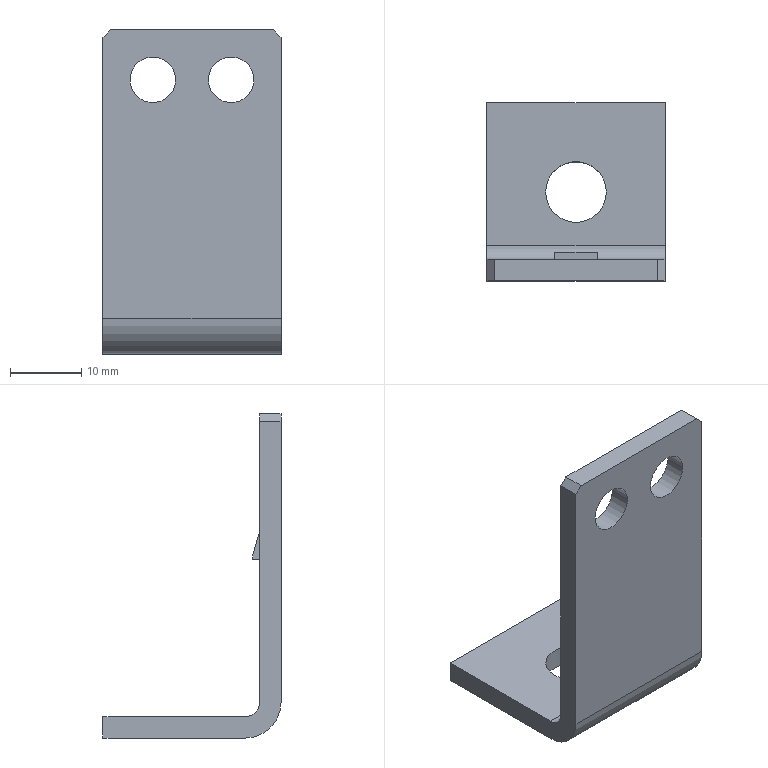Part | NX | features BREP 1 | 1 solid | 23 faces | box 25 x 25 x 45.51 mm | volume 4597 mm3 | plane 15 | cylinder 8 | commonest cylinder face diameters 6.4 x4 8.5 x2 4 x1 10 x1
STEP:
#1=CARTESIAN_POINT('',(15.241,-40.241,59.418));
#2=VERTEX_POINT('',#1);
#3=CARTESIAN_POINT('',(15.241,-37.241,59.418));
#4=VERTEX_POINT('',#3);
#5=CARTESIAN_POINT('',(15.241,-40.241,59.418));
#6=DIRECTION('',(0.,1.,0.));
#7=VECTOR('',#6,1000.);
#8=LINE('',#5,#7);
#9=EDGE_CURVE('',#2,#4,#8,.T.);
#10=ORIENTED_EDGE('',*,*,#9,.T.);
#11=CARTESIAN_POINT('',(15.241,-37.241,19.908));
#12=VERTEX_POINT('',#11);
#13=CARTESIAN_POINT('',(15.241,-37.241,19.908));
#14=DIRECTION('',(0.,0.,1.));
#15=VECTOR('',#14,1000.);
#16=LINE('',#13,#15);
#17=EDGE_CURVE('',#12,#4,#16,.T.);
#18=ORIENTED_EDGE('',*,*,#17,.F.);
#19=CARTESIAN_POINT('',(15.241,-35.241,17.908));
#20=VERTEX_POINT('',#19);
#21=CARTESIAN_POINT('',(15.241,-35.241,19.908));
#22=DIRECTION('',(1.,0.,0.));
#23=DIRECTION('',(0.,-1.,0.));
#24=AXIS2_PLACEMENT_3D('',#21,#22,#23);
#25=CIRCLE('',#24,2.);
#26=EDGE_CURVE('',#12,#20,#25,.T.);
#27=ORIENTED_EDGE('',*,*,#26,.T.);
#28=CARTESIAN_POINT('',(15.241,-15.241,17.908));
#29=VERTEX_POINT('',#28);
#30=CARTESIAN_POINT('',(15.241,-15.241,17.908));
#31=DIRECTION('',(0.,-1.,0.));
#32=VECTOR('',#31,1000.);
#33=LINE('',#30,#32);
#34=EDGE_CURVE('',#29,#20,#33,.T.);
#35=ORIENTED_EDGE('',*,*,#34,.F.);
#36=CARTESIAN_POINT('',(15.241,-15.241,14.908));
#37=VERTEX_POINT('',#36);
#38=CARTESIAN_POINT('',(15.241,-15.241,17.908));
#39=DIRECTION('',(0.,0.,-1.));
#40=VECTOR('',#39,1000.);
#41=LINE('',#38,#40);
#42=EDGE_CURVE('',#29,#37,#41,.T.);
#43=ORIENTED_EDGE('',*,*,#42,.T.);
#44=CARTESIAN_POINT('',(15.241,-35.241,14.908));
#45=VERTEX_POINT('',#44);
#46=CARTESIAN_POINT('',(15.241,-35.241,14.908));
#47=DIRECTION('',(0.,1.,0.));
#48=VECTOR('',#47,1000.);
#49=LINE('',#46,#48);
#50=EDGE_CURVE('',#45,#37,#49,.T.);
#51=ORIENTED_EDGE('',*,*,#50,.F.);
#52=CARTESIAN_POINT('',(15.241,-40.241,19.908));
#53=VERTEX_POINT('',#52);
#54=CARTESIAN_POINT('',(15.241,-35.241,19.908));
#55=DIRECTION('',(-1.,0.,0.));
#56=DIRECTION('',(0.,0.,-1.));
#57=AXIS2_PLACEMENT_3D('',#54,#55,#56);
#58=CIRCLE('',#57,5.);
#59=EDGE_CURVE('',#45,#53,#58,.T.);
#60=ORIENTED_EDGE('',*,*,#59,.T.);
#61=CARTESIAN_POINT('',(15.241,-40.241,59.418));
#62=DIRECTION('',(0.,0.,-1.));
#63=VECTOR('',#62,1000.);
#64=LINE('',#61,#63);
#65=EDGE_CURVE('',#2,#53,#64,.T.);
#66=ORIENTED_EDGE('',*,*,#65,.F.);
#67=EDGE_LOOP('',(#10,#18,#27,#35,#43,#51,#60,#66));
#68=FACE_BOUND('',#67,.T.);
#69=CARTESIAN_POINT('',(15.241,-37.241,19.226));
#70=DIRECTION('',(-1.,0.,0.));
#71=DIRECTION('',(0.,-1.,0.));
#72=AXIS2_PLACEMENT_3D('',#69,#70,#71);
#73=PLANE('',#72);
#74=ADVANCED_FACE('',(#68),#73,.T.);
#75=CARTESIAN_POINT('',(40.241,-40.241,59.418));
#76=VERTEX_POINT('',#75);
#77=CARTESIAN_POINT('',(39.241,-40.241,60.418));
#78=VERTEX_POINT('',#77);
#79=CARTESIAN_POINT('',(40.241,-40.241,59.418));
#80=DIRECTION('',(-0.7071,0.,0.7071));
#81=VECTOR('',#80,1000.);
#82=LINE('',#79,#81);
#83=EDGE_CURVE('',#76,#78,#82,.T.);
#84=ORIENTED_EDGE('',*,*,#83,.T.);
#85=CARTESIAN_POINT('',(16.241,-40.241,60.418));
#86=VERTEX_POINT('',#85);
#87=CARTESIAN_POINT('',(16.241,-40.241,60.418));
#88=DIRECTION('',(1.,0.,0.));
#89=VECTOR('',#88,1000.);
#90=LINE('',#87,#89);
#91=EDGE_CURVE('',#86,#78,#90,.T.);
#92=ORIENTED_EDGE('',*,*,#91,.F.);
#93=CARTESIAN_POINT('',(16.241,-40.241,60.418));
#94=DIRECTION('',(-0.7071,0.,-0.7071));
#95=VECTOR('',#94,1000.);
#96=LINE('',#93,#95);
#97=EDGE_CURVE('',#86,#2,#96,.T.);
#98=ORIENTED_EDGE('',*,*,#97,.T.);
#99=ORIENTED_EDGE('',*,*,#65,.T.);
#100=CARTESIAN_POINT('',(40.241,-40.241,19.908));
#101=VERTEX_POINT('',#100);
#102=CARTESIAN_POINT('',(40.241,-40.241,19.908));
#103=DIRECTION('',(-1.,0.,0.));
#104=VECTOR('',#103,1000.);
#105=LINE('',#102,#104);
#106=EDGE_CURVE('',#101,#53,#105,.T.);
#107=ORIENTED_EDGE('',*,*,#106,.F.);
#108=CARTESIAN_POINT('',(40.241,-40.241,59.418));
#109=DIRECTION('',(0.,0.,-1.));
#110=VECTOR('',#109,1000.);
#111=LINE('',#108,#110);
#112=EDGE_CURVE('',#76,#101,#111,.T.);
#113=ORIENTED_EDGE('',*,*,#112,.F.);
#114=EDGE_LOOP('',(#84,#92,#98,#99,#107,#113));
#115=FACE_BOUND('',#114,.T.);
#116=CARTESIAN_POINT('',(36.441,-40.241,53.418));
#117=VERTEX_POINT('',#116);
#118=CARTESIAN_POINT('',(30.041,-40.241,53.418));
#119=VERTEX_POINT('',#118);
#120=CARTESIAN_POINT('',(33.241,-40.241,53.418));
#121=DIRECTION('',(0.,1.,0.));
#122=DIRECTION('',(1.,0.,0.));
#123=AXIS2_PLACEMENT_3D('',#120,#121,#122);
#124=CIRCLE('',#123,3.2);
#125=EDGE_CURVE('',#117,#119,#124,.T.);
#126=ORIENTED_EDGE('',*,*,#125,.T.);
#127=CARTESIAN_POINT('',(33.241,-40.241,53.418));
#128=DIRECTION('',(0.,1.,0.));
#129=DIRECTION('',(-1.,0.,0.));
#130=AXIS2_PLACEMENT_3D('',#127,#128,#129);
#131=CIRCLE('',#130,3.2);
#132=EDGE_CURVE('',#119,#117,#131,.T.);
#133=ORIENTED_EDGE('',*,*,#132,.T.);
#134=EDGE_LOOP('',(#126,#133));
#135=FACE_BOUND('',#134,.T.);
#136=CARTESIAN_POINT('',(25.441,-40.241,53.418));
#137=VERTEX_POINT('',#136);
#138=CARTESIAN_POINT('',(19.041,-40.241,53.418));
#139=VERTEX_POINT('',#138);
#140=CARTESIAN_POINT('',(22.241,-40.241,53.418));
#141=DIRECTION('',(0.,1.,0.));
#142=DIRECTION('',(1.,0.,0.));
#143=AXIS2_PLACEMENT_3D('',#140,#141,#142);
#144=CIRCLE('',#143,3.2);
#145=EDGE_CURVE('',#137,#139,#144,.T.);
#146=ORIENTED_EDGE('',*,*,#145,.T.);
#147=CARTESIAN_POINT('',(22.241,-40.241,53.418));
#148=DIRECTION('',(0.,1.,0.));
#149=DIRECTION('',(-1.,0.,0.));
#150=AXIS2_PLACEMENT_3D('',#147,#148,#149);
#151=CIRCLE('',#150,3.2);
#152=EDGE_CURVE('',#139,#137,#151,.T.);
#153=ORIENTED_EDGE('',*,*,#152,.T.);
#154=EDGE_LOOP('',(#146,#153));
#155=FACE_BOUND('',#154,.T.);
#156=CARTESIAN_POINT('',(15.241,-40.241,19.226));
#157=DIRECTION('',(0.,-1.,0.));
#158=DIRECTION('',(1.,0.,0.));
#159=AXIS2_PLACEMENT_3D('',#156,#157,#158);
#160=PLANE('',#159);
#161=ADVANCED_FACE('',(#115,#135,#155),#160,.T.);
#162=CARTESIAN_POINT('',(40.241,-15.241,17.908));
#163=VERTEX_POINT('',#162);
#164=CARTESIAN_POINT('',(40.241,-15.241,14.908));
#165=VERTEX_POINT('',#164);
#166=CARTESIAN_POINT('',(40.241,-15.241,17.908));
#167=DIRECTION('',(0.,0.,-1.));
#168=VECTOR('',#167,1000.);
#169=LINE('',#166,#168);
#170=EDGE_CURVE('',#163,#165,#169,.T.);
#171=ORIENTED_EDGE('',*,*,#170,.F.);
#172=CARTESIAN_POINT('',(40.241,-35.241,17.908));
#173=VERTEX_POINT('',#172);
#174=CARTESIAN_POINT('',(40.241,-35.241,17.908));
#175=DIRECTION('',(0.,1.,0.));
#176=VECTOR('',#175,1000.);
#177=LINE('',#174,#176);
#178=EDGE_CURVE('',#173,#163,#177,.T.);
#179=ORIENTED_EDGE('',*,*,#178,.F.);
#180=CARTESIAN_POINT('',(40.241,-37.241,19.908));
#181=VERTEX_POINT('',#180);
#182=CARTESIAN_POINT('',(40.241,-35.241,19.908));
#183=DIRECTION('',(-1.,0.,0.));
#184=DIRECTION('',(0.,0.,-1.));
#185=AXIS2_PLACEMENT_3D('',#182,#183,#184);
#186=CIRCLE('',#185,2.);
#187=EDGE_CURVE('',#173,#181,#186,.T.);
#188=ORIENTED_EDGE('',*,*,#187,.T.);
#189=CARTESIAN_POINT('',(40.241,-37.241,59.418));
#190=VERTEX_POINT('',#189);
#191=CARTESIAN_POINT('',(40.241,-37.241,59.418));
#192=DIRECTION('',(0.,0.,-1.));
#193=VECTOR('',#192,1000.);
#194=LINE('',#191,#193);
#195=EDGE_CURVE('',#190,#181,#194,.T.);
#196=ORIENTED_EDGE('',*,*,#195,.F.);
#197=CARTESIAN_POINT('',(40.241,-37.241,59.418));
#198=DIRECTION('',(0.,-1.,0.));
#199=VECTOR('',#198,1000.);
#200=LINE('',#197,#199);
#201=EDGE_CURVE('',#190,#76,#200,.T.);
#202=ORIENTED_EDGE('',*,*,#201,.T.);
#203=ORIENTED_EDGE('',*,*,#112,.T.);
#204=CARTESIAN_POINT('',(40.241,-35.241,14.908));
#205=VERTEX_POINT('',#204);
#206=CARTESIAN_POINT('',(40.241,-35.241,19.908));
#207=DIRECTION('',(1.,0.,0.));
#208=DIRECTION('',(0.,-1.,0.));
#209=AXIS2_PLACEMENT_3D('',#206,#207,#208);
#210=CIRCLE('',#209,5.);
#211=EDGE_CURVE('',#101,#205,#210,.T.);
#212=ORIENTED_EDGE('',*,*,#211,.T.);
#213=CARTESIAN_POINT('',(40.241,-15.241,14.908));
#214=DIRECTION('',(0.,-1.,0.));
#215=VECTOR('',#214,1000.);
#216=LINE('',#213,#215);
#217=EDGE_CURVE('',#165,#205,#216,.T.);
#218=ORIENTED_EDGE('',*,*,#217,.F.);
#219=EDGE_LOOP('',(#171,#179,#188,#196,#202,#203,#212,#218));
#220=FACE_BOUND('',#219,.T.);
#221=CARTESIAN_POINT('',(40.241,-40.241,19.226));
#222=DIRECTION('',(1.,0.,0.));
#223=DIRECTION('',(0.,1.,0.));
#224=AXIS2_PLACEMENT_3D('',#221,#222,#223);
#225=PLANE('',#224);
#226=ADVANCED_FACE('',(#220),#225,.T.);
#227=CARTESIAN_POINT('',(15.241,-15.241,14.908));
#228=DIRECTION('',(1.,0.,0.));
#229=VECTOR('',#228,1000.);
#230=LINE('',#227,#229);
#231=EDGE_CURVE('',#37,#165,#230,.T.);
#232=ORIENTED_EDGE('',*,*,#231,.T.);
#233=ORIENTED_EDGE('',*,*,#217,.T.);
#234=CARTESIAN_POINT('',(15.241,-35.241,14.908));
#235=DIRECTION('',(1.,0.,0.));
#236=VECTOR('',#235,1000.);
#237=LINE('',#234,#236);
#238=EDGE_CURVE('',#45,#205,#237,.T.);
#239=ORIENTED_EDGE('',*,*,#238,.F.);
#240=ORIENTED_EDGE('',*,*,#50,.T.);
#241=EDGE_LOOP('',(#232,#233,#239,#240));
#242=FACE_BOUND('',#241,.T.);
#243=CARTESIAN_POINT('',(31.991,-27.741,14.908));
#244=VERTEX_POINT('',#243);
#245=CARTESIAN_POINT('',(23.491,-27.741,14.908));
#246=VERTEX_POINT('',#245);
#247=CARTESIAN_POINT('',(27.741,-27.741,14.908));
#248=DIRECTION('',(0.,0.,1.));
#249=DIRECTION('',(1.,0.,0.));
#250=AXIS2_PLACEMENT_3D('',#247,#248,#249);
#251=CIRCLE('',#250,4.25);
#252=EDGE_CURVE('',#244,#246,#251,.T.);
#253=ORIENTED_EDGE('',*,*,#252,.T.);
#254=CARTESIAN_POINT('',(27.741,-27.741,14.908));
#255=DIRECTION('',(0.,0.,1.));
#256=DIRECTION('',(-1.,0.,0.));
#257=AXIS2_PLACEMENT_3D('',#254,#255,#256);
#258=CIRCLE('',#257,4.25);
#259=EDGE_CURVE('',#246,#244,#258,.T.);
#260=ORIENTED_EDGE('',*,*,#259,.T.);
#261=EDGE_LOOP('',(#253,#260));
#262=FACE_BOUND('',#261,.T.);
#263=CARTESIAN_POINT('',(0.,0.,14.908));
#264=DIRECTION('',(0.,0.,-1.));
#265=DIRECTION('',(-1.,0.,0.));
#266=AXIS2_PLACEMENT_3D('',#263,#264,#265);
#267=PLANE('',#266);
#268=ADVANCED_FACE('',(#242,#262),#267,.T.);
#269=ORIENTED_EDGE('',*,*,#211,.F.);
#270=ORIENTED_EDGE('',*,*,#106,.T.);
#271=ORIENTED_EDGE('',*,*,#59,.F.);
#272=ORIENTED_EDGE('',*,*,#238,.T.);
#273=EDGE_LOOP('',(#269,#270,#271,#272));
#274=FACE_BOUND('',#273,.T.);
#275=CARTESIAN_POINT('',(72.831,-35.241,19.908));
#276=DIRECTION('',(-1.,0.,0.));
#277=DIRECTION('',(0.,0.,-1.));
#278=AXIS2_PLACEMENT_3D('',#275,#276,#277);
#279=CYLINDRICAL_SURFACE('',#278,5.);
#280=ADVANCED_FACE('',(#274),#279,.T.);
#281=ORIENTED_EDGE('',*,*,#231,.F.);
#282=ORIENTED_EDGE('',*,*,#42,.F.);
#283=CARTESIAN_POINT('',(15.241,-15.241,17.908));
#284=DIRECTION('',(1.,0.,0.));
#285=VECTOR('',#284,1000.);
#286=LINE('',#283,#285);
#287=EDGE_CURVE('',#29,#163,#286,.T.);
#288=ORIENTED_EDGE('',*,*,#287,.T.);
#289=ORIENTED_EDGE('',*,*,#170,.T.);
#290=EDGE_LOOP('',(#281,#282,#288,#289));
#291=FACE_BOUND('',#290,.T.);
#292=CARTESIAN_POINT('',(15.241,-15.241,20.908));
#293=DIRECTION('',(0.,1.,0.));
#294=DIRECTION('',(1.,0.,0.));
#295=AXIS2_PLACEMENT_3D('',#292,#293,#294);
#296=PLANE('',#295);
#297=ADVANCED_FACE('',(#291),#296,.T.);
#298=ORIENTED_EDGE('',*,*,#287,.F.);
#299=ORIENTED_EDGE('',*,*,#34,.T.);
#300=CARTESIAN_POINT('',(40.241,-35.241,17.908));
#301=DIRECTION('',(-1.,0.,0.));
#302=VECTOR('',#301,1000.);
#303=LINE('',#300,#302);
#304=EDGE_CURVE('',#173,#20,#303,.T.);
#305=ORIENTED_EDGE('',*,*,#304,.F.);
#306=ORIENTED_EDGE('',*,*,#178,.T.);
#307=EDGE_LOOP('',(#298,#299,#305,#306));
#308=FACE_BOUND('',#307,.T.);
#309=CARTESIAN_POINT('',(23.491,-27.741,17.908));
#310=VERTEX_POINT('',#309);
#311=CARTESIAN_POINT('',(31.991,-27.741,17.908));
#312=VERTEX_POINT('',#311);
#313=CARTESIAN_POINT('',(27.741,-27.741,17.908));
#314=DIRECTION('',(0.,0.,-1.));
#315=DIRECTION('',(-1.,0.,0.));
#316=AXIS2_PLACEMENT_3D('',#313,#314,#315);
#317=CIRCLE('',#316,4.25);
#318=EDGE_CURVE('',#310,#312,#317,.T.);
#319=ORIENTED_EDGE('',*,*,#318,.T.);
#320=CARTESIAN_POINT('',(27.741,-27.741,17.908));
#321=DIRECTION('',(0.,0.,-1.));
#322=DIRECTION('',(1.,0.,0.));
#323=AXIS2_PLACEMENT_3D('',#320,#321,#322);
#324=CIRCLE('',#323,4.25);
#325=EDGE_CURVE('',#312,#310,#324,.T.);
#326=ORIENTED_EDGE('',*,*,#325,.T.);
#327=EDGE_LOOP('',(#319,#326));
#328=FACE_BOUND('',#327,.T.);
#329=CARTESIAN_POINT('',(0.,0.,17.908));
#330=DIRECTION('',(0.,0.,-1.));
#331=DIRECTION('',(-1.,0.,0.));
#332=AXIS2_PLACEMENT_3D('',#329,#330,#331);
#333=PLANE('',#332);
#334=ADVANCED_FACE('',(#308,#328),#333,.F.);
#335=ORIENTED_EDGE('',*,*,#304,.T.);
#336=ORIENTED_EDGE('',*,*,#26,.F.);
#337=CARTESIAN_POINT('',(15.241,-37.241,19.908));
#338=DIRECTION('',(1.,0.,0.));
#339=VECTOR('',#338,1000.);
#340=LINE('',#337,#339);
#341=EDGE_CURVE('',#12,#181,#340,.T.);
#342=ORIENTED_EDGE('',*,*,#341,.T.);
#343=ORIENTED_EDGE('',*,*,#187,.F.);
#344=EDGE_LOOP('',(#335,#336,#342,#343));
#345=FACE_BOUND('',#344,.T.);
#346=CARTESIAN_POINT('',(-17.349,-35.241,19.908));
#347=DIRECTION('',(1.,0.,0.));
#348=DIRECTION('',(0.,-1.,0.));
#349=AXIS2_PLACEMENT_3D('',#346,#347,#348);
#350=CYLINDRICAL_SURFACE('',#349,2.);
#351=ADVANCED_FACE('',(#345),#350,.F.);
#352=CARTESIAN_POINT('',(16.241,-37.241,60.418));
#353=VERTEX_POINT('',#352);
#354=CARTESIAN_POINT('',(15.241,-37.241,59.418));
#355=DIRECTION('',(0.7071,0.,0.7071));
#356=VECTOR('',#355,1000.);
#357=LINE('',#354,#356);
#358=EDGE_CURVE('',#4,#353,#357,.T.);
#359=ORIENTED_EDGE('',*,*,#358,.T.);
#360=CARTESIAN_POINT('',(39.241,-37.241,60.418));
#361=VERTEX_POINT('',#360);
#362=CARTESIAN_POINT('',(39.241,-37.241,60.418));
#363=DIRECTION('',(-1.,0.,0.));
#364=VECTOR('',#363,1000.);
#365=LINE('',#362,#364);
#366=EDGE_CURVE('',#361,#353,#365,.T.);
#367=ORIENTED_EDGE('',*,*,#366,.F.);
#368=CARTESIAN_POINT('',(39.241,-37.241,60.418));
#369=DIRECTION('',(0.7071,0.,-0.7071));
#370=VECTOR('',#369,1000.);
#371=LINE('',#368,#370);
#372=EDGE_CURVE('',#361,#190,#371,.T.);
#373=ORIENTED_EDGE('',*,*,#372,.T.);
#374=ORIENTED_EDGE('',*,*,#195,.T.);
#375=ORIENTED_EDGE('',*,*,#341,.F.);
#376=ORIENTED_EDGE('',*,*,#17,.T.);
#377=EDGE_LOOP('',(#359,#367,#373,#374,#375,#376));
#378=FACE_BOUND('',#377,.T.);
#379=CARTESIAN_POINT('',(30.741,-37.241,40.026));
#380=VERTEX_POINT('',#379);
#381=CARTESIAN_POINT('',(30.741,-37.241,43.882));
#382=VERTEX_POINT('',#381);
#383=CARTESIAN_POINT('',(30.741,-37.241,40.026));
#384=DIRECTION('',(0.,0.,1.));
#385=VECTOR('',#384,1000.);
#386=LINE('',#383,#385);
#387=EDGE_CURVE('',#380,#382,#386,.T.);
#388=ORIENTED_EDGE('',*,*,#387,.T.);
#389=CARTESIAN_POINT('',(24.741,-37.241,43.882));
#390=VERTEX_POINT('',#389);
#391=CARTESIAN_POINT('',(24.741,-37.241,43.882));
#392=DIRECTION('',(1.,0.,0.));
#393=VECTOR('',#392,1000.);
#394=LINE('',#391,#393);
#395=EDGE_CURVE('',#390,#382,#394,.T.);
#396=ORIENTED_EDGE('',*,*,#395,.F.);
#397=CARTESIAN_POINT('',(24.741,-37.241,40.026));
#398=VERTEX_POINT('',#397);
#399=CARTESIAN_POINT('',(24.741,-37.241,43.882));
#400=DIRECTION('',(0.,0.,-1.));
#401=VECTOR('',#400,1000.);
#402=LINE('',#399,#401);
#403=EDGE_CURVE('',#390,#398,#402,.T.);
#404=ORIENTED_EDGE('',*,*,#403,.T.);
#405=CARTESIAN_POINT('',(30.741,-37.241,40.026));
#406=DIRECTION('',(-1.,0.,0.));
#407=VECTOR('',#406,1000.);
#408=LINE('',#405,#407);
#409=EDGE_CURVE('',#380,#398,#408,.T.);
#410=ORIENTED_EDGE('',*,*,#409,.F.);
#411=EDGE_LOOP('',(#388,#396,#404,#410));
#412=FACE_BOUND('',#411,.T.);
#413=CARTESIAN_POINT('',(36.441,-37.241,53.418));
#414=VERTEX_POINT('',#413);
#415=CARTESIAN_POINT('',(30.041,-37.241,53.418));
#416=VERTEX_POINT('',#415);
#417=CARTESIAN_POINT('',(33.241,-37.241,53.418));
#418=DIRECTION('',(0.,1.,0.));
#419=DIRECTION('',(1.,0.,0.));
#420=AXIS2_PLACEMENT_3D('',#417,#418,#419);
#421=CIRCLE('',#420,3.2);
#422=EDGE_CURVE('',#414,#416,#421,.T.);
#423=ORIENTED_EDGE('',*,*,#422,.F.);
#424=CARTESIAN_POINT('',(33.241,-37.241,53.418));
#425=DIRECTION('',(0.,1.,0.));
#426=DIRECTION('',(-1.,0.,0.));
#427=AXIS2_PLACEMENT_3D('',#424,#425,#426);
#428=CIRCLE('',#427,3.2);
#429=EDGE_CURVE('',#416,#414,#428,.T.);
#430=ORIENTED_EDGE('',*,*,#429,.F.);
#431=EDGE_LOOP('',(#423,#430));
#432=FACE_BOUND('',#431,.T.);
#433=CARTESIAN_POINT('',(25.441,-37.241,53.418));
#434=VERTEX_POINT('',#433);
#435=CARTESIAN_POINT('',(19.041,-37.241,53.418));
#436=VERTEX_POINT('',#435);
#437=CARTESIAN_POINT('',(22.241,-37.241,53.418));
#438=DIRECTION('',(0.,1.,0.));
#439=DIRECTION('',(1.,0.,0.));
#440=AXIS2_PLACEMENT_3D('',#437,#438,#439);
#441=CIRCLE('',#440,3.2);
#442=EDGE_CURVE('',#434,#436,#441,.T.);
#443=ORIENTED_EDGE('',*,*,#442,.F.);
#444=CARTESIAN_POINT('',(22.241,-37.241,53.418));
#445=DIRECTION('',(0.,1.,0.));
#446=DIRECTION('',(-1.,0.,0.));
#447=AXIS2_PLACEMENT_3D('',#444,#445,#446);
#448=CIRCLE('',#447,3.2);
#449=EDGE_CURVE('',#436,#434,#448,.T.);
#450=ORIENTED_EDGE('',*,*,#449,.F.);
#451=EDGE_LOOP('',(#443,#450));
#452=FACE_BOUND('',#451,.T.);
#453=CARTESIAN_POINT('',(40.241,-37.241,19.226));
#454=DIRECTION('',(0.,1.,0.));
#455=DIRECTION('',(-1.,0.,0.));
#456=AXIS2_PLACEMENT_3D('',#453,#454,#455);
#457=PLANE('',#456);
#458=ADVANCED_FACE('',(#378,#412,#432,#452),#457,.T.);
#459=ORIENTED_EDGE('',*,*,#372,.F.);
#460=CARTESIAN_POINT('',(39.241,-37.241,60.418));
#461=DIRECTION('',(0.,-1.,0.));
#462=VECTOR('',#461,1000.);
#463=LINE('',#460,#462);
#464=EDGE_CURVE('',#361,#78,#463,.T.);
#465=ORIENTED_EDGE('',*,*,#464,.T.);
#466=ORIENTED_EDGE('',*,*,#83,.F.);
#467=ORIENTED_EDGE('',*,*,#201,.F.);
#468=EDGE_LOOP('',(#459,#465,#466,#467));
#469=FACE_BOUND('',#468,.T.);
#470=CARTESIAN_POINT('',(39.741,-38.741,59.918));
#471=DIRECTION('',(0.7071,0.,0.7071));
#472=DIRECTION('',(-0.7071,0.,0.7071));
#473=AXIS2_PLACEMENT_3D('',#470,#471,#472);
#474=PLANE('',#473);
#475=ADVANCED_FACE('',(#469),#474,.T.);
#476=CARTESIAN_POINT('',(16.241,-40.241,60.418));
#477=DIRECTION('',(0.,1.,0.));
#478=VECTOR('',#477,1000.);
#479=LINE('',#476,#478);
#480=EDGE_CURVE('',#86,#353,#479,.T.);
#481=ORIENTED_EDGE('',*,*,#480,.F.);
#482=ORIENTED_EDGE('',*,*,#91,.T.);
#483=ORIENTED_EDGE('',*,*,#464,.F.);
#484=ORIENTED_EDGE('',*,*,#366,.T.);
#485=EDGE_LOOP('',(#481,#482,#483,#484));
#486=FACE_BOUND('',#485,.T.);
#487=CARTESIAN_POINT('',(0.,0.,60.418));
#488=DIRECTION('',(0.,0.,1.));
#489=DIRECTION('',(1.,0.,0.));
#490=AXIS2_PLACEMENT_3D('',#487,#488,#489);
#491=PLANE('',#490);
#492=ADVANCED_FACE('',(#486),#491,.T.);
#493=ORIENTED_EDGE('',*,*,#97,.F.);
#494=ORIENTED_EDGE('',*,*,#480,.T.);
#495=ORIENTED_EDGE('',*,*,#358,.F.);
#496=ORIENTED_EDGE('',*,*,#9,.F.);
#497=EDGE_LOOP('',(#493,#494,#495,#496));
#498=FACE_BOUND('',#497,.T.);
#499=CARTESIAN_POINT('',(15.741,-38.741,59.918));
#500=DIRECTION('',(-0.7071,0.,0.7071));
#501=DIRECTION('',(0.7071,0.,0.7071));
#502=AXIS2_PLACEMENT_3D('',#499,#500,#501);
#503=PLANE('',#502);
#504=ADVANCED_FACE('',(#498),#503,.T.);
#505=CARTESIAN_POINT('',(24.741,-36.241,40.026));
#506=VERTEX_POINT('',#505);
#507=CARTESIAN_POINT('',(24.741,-37.241,40.026));
#508=DIRECTION('',(0.,1.,0.));
#509=VECTOR('',#508,1000.);
#510=LINE('',#507,#509);
#511=EDGE_CURVE('',#398,#506,#510,.T.);
#512=ORIENTED_EDGE('',*,*,#511,.T.);
#513=CARTESIAN_POINT('',(30.741,-36.241,40.026));
#514=VERTEX_POINT('',#513);
#515=CARTESIAN_POINT('',(30.741,-36.241,40.026));
#516=DIRECTION('',(-1.,0.,0.));
#517=VECTOR('',#516,1000.);
#518=LINE('',#515,#517);
#519=EDGE_CURVE('',#514,#506,#518,.T.);
#520=ORIENTED_EDGE('',*,*,#519,.F.);
#521=CARTESIAN_POINT('',(30.741,-37.241,40.026));
#522=DIRECTION('',(0.,1.,0.));
#523=VECTOR('',#522,1000.);
#524=LINE('',#521,#523);
#525=EDGE_CURVE('',#380,#514,#524,.T.);
#526=ORIENTED_EDGE('',*,*,#525,.F.);
#527=ORIENTED_EDGE('',*,*,#409,.T.);
#528=EDGE_LOOP('',(#512,#520,#526,#527));
#529=FACE_BOUND('',#528,.T.);
#530=CARTESIAN_POINT('',(24.741,-37.241,40.026));
#531=DIRECTION('',(0.,0.,-1.));
#532=DIRECTION('',(0.,1.,0.));
#533=AXIS2_PLACEMENT_3D('',#530,#531,#532);
#534=PLANE('',#533);
#535=ADVANCED_FACE('',(#529),#534,.T.);
#536=ORIENTED_EDGE('',*,*,#387,.F.);
#537=ORIENTED_EDGE('',*,*,#525,.T.);
#538=CARTESIAN_POINT('',(30.741,-36.241,40.482));
#539=VERTEX_POINT('',#538);
#540=CARTESIAN_POINT('',(30.741,-36.241,40.482));
#541=DIRECTION('',(0.,0.,-1.));
#542=VECTOR('',#541,1000.);
#543=LINE('',#540,#542);
#544=EDGE_CURVE('',#539,#514,#543,.T.);
#545=ORIENTED_EDGE('',*,*,#544,.F.);
#546=CARTESIAN_POINT('',(30.741,-36.241,40.482));
#547=DIRECTION('',(0.,-0.2822,0.9594));
#548=VECTOR('',#547,1000.);
#549=LINE('',#546,#548);
#550=EDGE_CURVE('',#539,#382,#549,.T.);
#551=ORIENTED_EDGE('',*,*,#550,.T.);
#552=EDGE_LOOP('',(#536,#537,#545,#551));
#553=FACE_BOUND('',#552,.T.);
#554=CARTESIAN_POINT('',(30.741,0.,35.426));
#555=DIRECTION('',(1.,0.,0.));
#556=DIRECTION('',(0.,1.,0.));
#557=AXIS2_PLACEMENT_3D('',#554,#555,#556);
#558=PLANE('',#557);
#559=ADVANCED_FACE('',(#553),#558,.T.);
#560=CARTESIAN_POINT('',(24.741,-36.241,40.482));
#561=VERTEX_POINT('',#560);
#562=CARTESIAN_POINT('',(24.741,-37.241,43.882));
#563=DIRECTION('',(0.,0.2822,-0.9594));
#564=VECTOR('',#563,1000.);
#565=LINE('',#562,#564);
#566=EDGE_CURVE('',#390,#561,#565,.T.);
#567=ORIENTED_EDGE('',*,*,#566,.F.);
#568=ORIENTED_EDGE('',*,*,#395,.T.);
#569=ORIENTED_EDGE('',*,*,#550,.F.);
#570=CARTESIAN_POINT('',(30.741,-36.241,40.482));
#571=DIRECTION('',(-1.,0.,0.));
#572=VECTOR('',#571,1000.);
#573=LINE('',#570,#572);
#574=EDGE_CURVE('',#539,#561,#573,.T.);
#575=ORIENTED_EDGE('',*,*,#574,.T.);
#576=EDGE_LOOP('',(#567,#568,#569,#575));
#577=FACE_BOUND('',#576,.T.);
#578=CARTESIAN_POINT('',(24.741,-37.201,43.743));
#579=DIRECTION('',(0.,0.9594,0.2822));
#580=DIRECTION('',(0.,-0.2822,0.9594));
#581=AXIS2_PLACEMENT_3D('',#578,#579,#580);
#582=PLANE('',#581);
#583=ADVANCED_FACE('',(#577),#582,.T.);
#584=ORIENTED_EDGE('',*,*,#544,.T.);
#585=ORIENTED_EDGE('',*,*,#519,.T.);
#586=CARTESIAN_POINT('',(24.741,-36.241,40.482));
#587=DIRECTION('',(0.,0.,-1.));
#588=VECTOR('',#587,1000.);
#589=LINE('',#586,#588);
#590=EDGE_CURVE('',#561,#506,#589,.T.);
#591=ORIENTED_EDGE('',*,*,#590,.F.);
#592=ORIENTED_EDGE('',*,*,#574,.F.);
#593=EDGE_LOOP('',(#584,#585,#591,#592));
#594=FACE_BOUND('',#593,.T.);
#595=CARTESIAN_POINT('',(27.741,-36.241,42.026));
#596=DIRECTION('',(0.,1.,0.));
#597=DIRECTION('',(1.,0.,0.));
#598=AXIS2_PLACEMENT_3D('',#595,#596,#597);
#599=PLANE('',#598);
#600=ADVANCED_FACE('',(#594),#599,.T.);
#601=ORIENTED_EDGE('',*,*,#566,.T.);
#602=ORIENTED_EDGE('',*,*,#590,.T.);
#603=ORIENTED_EDGE('',*,*,#511,.F.);
#604=ORIENTED_EDGE('',*,*,#403,.F.);
#605=EDGE_LOOP('',(#601,#602,#603,#604));
#606=FACE_BOUND('',#605,.T.);
#607=CARTESIAN_POINT('',(24.741,0.,35.426));
#608=DIRECTION('',(1.,0.,0.));
#609=DIRECTION('',(0.,1.,0.));
#610=AXIS2_PLACEMENT_3D('',#607,#608,#609);
#611=PLANE('',#610);
#612=ADVANCED_FACE('',(#606),#611,.F.);
#613=CARTESIAN_POINT('',(30.041,-37.241,53.418));
#614=DIRECTION('',(0.,1.,0.));
#615=VECTOR('',#614,1000.);
#616=LINE('',#613,#615);
#617=EDGE_CURVE('',#119,#416,#616,.T.);
#618=ORIENTED_EDGE('',*,*,#617,.T.);
#619=ORIENTED_EDGE('',*,*,#429,.T.);
#620=CARTESIAN_POINT('',(36.441,-37.241,53.418));
#621=DIRECTION('',(0.,1.,0.));
#622=VECTOR('',#621,1000.);
#623=LINE('',#620,#622);
#624=EDGE_CURVE('',#117,#414,#623,.T.);
#625=ORIENTED_EDGE('',*,*,#624,.F.);
#626=ORIENTED_EDGE('',*,*,#132,.F.);
#627=EDGE_LOOP('',(#618,#619,#625,#626));
#628=FACE_BOUND('',#627,.T.);
#629=CARTESIAN_POINT('',(33.241,-37.241,53.418));
#630=DIRECTION('',(0.,1.,0.));
#631=DIRECTION('',(1.,0.,0.));
#632=AXIS2_PLACEMENT_3D('',#629,#630,#631);
#633=CYLINDRICAL_SURFACE('',#632,3.2);
#634=ADVANCED_FACE('',(#628),#633,.F.);
#635=ORIENTED_EDGE('',*,*,#624,.T.);
#636=ORIENTED_EDGE('',*,*,#422,.T.);
#637=ORIENTED_EDGE('',*,*,#617,.F.);
#638=ORIENTED_EDGE('',*,*,#125,.F.);
#639=EDGE_LOOP('',(#635,#636,#637,#638));
#640=FACE_BOUND('',#639,.T.);
#641=CARTESIAN_POINT('',(33.241,-37.241,53.418));
#642=DIRECTION('',(0.,1.,0.));
#643=DIRECTION('',(1.,0.,0.));
#644=AXIS2_PLACEMENT_3D('',#641,#642,#643);
#645=CYLINDRICAL_SURFACE('',#644,3.2);
#646=ADVANCED_FACE('',(#640),#645,.F.);
#647=CARTESIAN_POINT('',(19.041,-37.241,53.418));
#648=DIRECTION('',(0.,1.,0.));
#649=VECTOR('',#648,1000.);
#650=LINE('',#647,#649);
#651=EDGE_CURVE('',#139,#436,#650,.T.);
#652=ORIENTED_EDGE('',*,*,#651,.T.);
#653=ORIENTED_EDGE('',*,*,#449,.T.);
#654=CARTESIAN_POINT('',(25.441,-37.241,53.418));
#655=DIRECTION('',(0.,1.,0.));
#656=VECTOR('',#655,1000.);
#657=LINE('',#654,#656);
#658=EDGE_CURVE('',#137,#434,#657,.T.);
#659=ORIENTED_EDGE('',*,*,#658,.F.);
#660=ORIENTED_EDGE('',*,*,#152,.F.);
#661=EDGE_LOOP('',(#652,#653,#659,#660));
#662=FACE_BOUND('',#661,.T.);
#663=CARTESIAN_POINT('',(22.241,-37.241,53.418));
#664=DIRECTION('',(0.,1.,0.));
#665=DIRECTION('',(1.,0.,0.));
#666=AXIS2_PLACEMENT_3D('',#663,#664,#665);
#667=CYLINDRICAL_SURFACE('',#666,3.2);
#668=ADVANCED_FACE('',(#662),#667,.F.);
#669=ORIENTED_EDGE('',*,*,#658,.T.);
#670=ORIENTED_EDGE('',*,*,#442,.T.);
#671=ORIENTED_EDGE('',*,*,#651,.F.);
#672=ORIENTED_EDGE('',*,*,#145,.F.);
#673=EDGE_LOOP('',(#669,#670,#671,#672));
#674=FACE_BOUND('',#673,.T.);
#675=CARTESIAN_POINT('',(22.241,-37.241,53.418));
#676=DIRECTION('',(0.,1.,0.));
#677=DIRECTION('',(1.,0.,0.));
#678=AXIS2_PLACEMENT_3D('',#675,#676,#677);
#679=CYLINDRICAL_SURFACE('',#678,3.2);
#680=ADVANCED_FACE('',(#674),#679,.F.);
#681=ORIENTED_EDGE('',*,*,#259,.F.);
#682=CARTESIAN_POINT('',(23.491,-27.741,14.908));
#683=DIRECTION('',(0.,0.,1.));
#684=VECTOR('',#683,1000.);
#685=LINE('',#682,#684);
#686=EDGE_CURVE('',#246,#310,#685,.T.);
#687=ORIENTED_EDGE('',*,*,#686,.T.);
#688=ORIENTED_EDGE('',*,*,#325,.F.);
#689=CARTESIAN_POINT('',(31.991,-27.741,14.908));
#690=DIRECTION('',(0.,0.,1.));
#691=VECTOR('',#690,1000.);
#692=LINE('',#689,#691);
#693=EDGE_CURVE('',#244,#312,#692,.T.);
#694=ORIENTED_EDGE('',*,*,#693,.F.);
#695=EDGE_LOOP('',(#681,#687,#688,#694));
#696=FACE_BOUND('',#695,.T.);
#697=CARTESIAN_POINT('',(27.741,-27.741,17.908));
#698=DIRECTION('',(0.,0.,-1.));
#699=DIRECTION('',(-1.,0.,0.));
#700=AXIS2_PLACEMENT_3D('',#697,#698,#699);
#701=CYLINDRICAL_SURFACE('',#700,4.25);
#702=ADVANCED_FACE('',(#696),#701,.F.);
#703=ORIENTED_EDGE('',*,*,#252,.F.);
#704=ORIENTED_EDGE('',*,*,#693,.T.);
#705=ORIENTED_EDGE('',*,*,#318,.F.);
#706=ORIENTED_EDGE('',*,*,#686,.F.);
#707=EDGE_LOOP('',(#703,#704,#705,#706));
#708=FACE_BOUND('',#707,.T.);
#709=CARTESIAN_POINT('',(27.741,-27.741,17.908));
#710=DIRECTION('',(0.,0.,-1.));
#711=DIRECTION('',(-1.,0.,0.));
#712=AXIS2_PLACEMENT_3D('',#709,#710,#711);
#713=CYLINDRICAL_SURFACE('',#712,4.25);
#714=ADVANCED_FACE('',(#708),#713,.F.);
#715=CLOSED_SHELL('',(#74,#161,#226,#268,#280,#297,#334,#351,#458,#475,#492,#504,#535,#559,#583,#600,#612,#634,#646,#668,#680,#702,#714));
#716=MANIFOLD_SOLID_BREP('',#715);
#717=(LENGTH_UNIT()NAMED_UNIT(*)SI_UNIT(.MILLI.,.METRE.));
#718=UNCERTAINTY_MEASURE_WITH_UNIT(LENGTH_MEASURE(0.00001),#717,'','');
#719=(NAMED_UNIT(*)PLANE_ANGLE_UNIT()SI_UNIT($,.RADIAN.));
#720=(NAMED_UNIT(*)SI_UNIT($,.STERADIAN.)SOLID_ANGLE_UNIT());
#721=(GEOMETRIC_REPRESENTATION_CONTEXT(3)GLOBAL_UNCERTAINTY_ASSIGNED_CONTEXT((#718))GLOBAL_UNIT_ASSIGNED_CONTEXT((#717,#719,#720))REPRESENTATION_CONTEXT('',''));
#722=ADVANCED_BREP_SHAPE_REPRESENTATION('',(#716),#721);